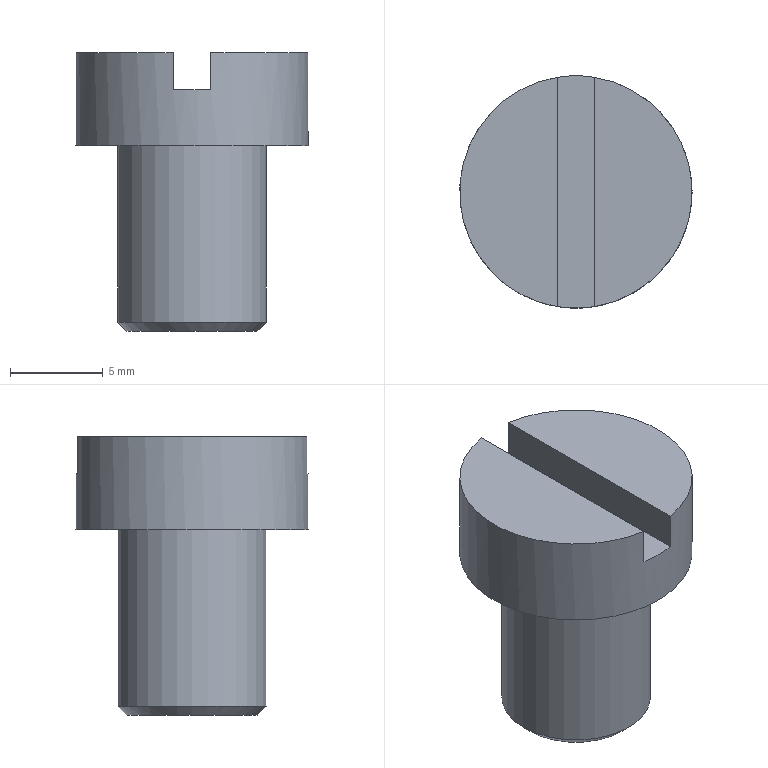Part | NX | features DATUM_CSYS 4, EXTRUDE 3, SKETCH 3, CHAMFER 1 | 1 solid | 10 faces | box 12.5 x 12.5 x 15 mm | volume 1063 mm3 | plane 7 | cylinder 2 | cone 1 | commonest cylinder face diameters 8 x1 12.5 x1
STEP:
#1=CARTESIAN_POINT('',(-1.,6.169,5.));
#2=VERTEX_POINT('',#1);
#3=CARTESIAN_POINT('',(-1.,-6.169,5.));
#4=VERTEX_POINT('',#3);
#5=CARTESIAN_POINT('',(-1.,13.407,5.));
#6=DIRECTION('',(0.,-1.,0.));
#7=VECTOR('',#6,1000.);
#8=LINE('',#5,#7);
#9=EDGE_CURVE('',#2,#4,#8,.T.);
#10=ORIENTED_EDGE('',*,*,#9,.F.);
#11=CARTESIAN_POINT('',(0.,0.,5.));
#12=DIRECTION('',(0.,0.,1.));
#13=DIRECTION('',(1.,0.,0.));
#14=AXIS2_PLACEMENT_3D('',#11,#12,#13);
#15=CIRCLE('',#14,6.25);
#16=EDGE_CURVE('',#2,#4,#15,.T.);
#17=ORIENTED_EDGE('',*,*,#16,.T.);
#18=EDGE_LOOP('',(#10,#17));
#19=FACE_BOUND('',#18,.T.);
#20=CARTESIAN_POINT('',(0.,0.,5.));
#21=DIRECTION('',(0.,0.,1.));
#22=DIRECTION('',(1.,0.,0.));
#23=AXIS2_PLACEMENT_3D('',#20,#21,#22);
#24=PLANE('',#23);
#25=ADVANCED_FACE('',(#19),#24,.T.);
#26=ORIENTED_EDGE('',*,*,#16,.F.);
#27=CARTESIAN_POINT('',(-1.,6.169,3.));
#28=VERTEX_POINT('',#27);
#29=CARTESIAN_POINT('',(-1.,6.169,5.));
#30=DIRECTION('',(0.,0.,-1.));
#31=VECTOR('',#30,1000.);
#32=LINE('',#29,#31);
#33=EDGE_CURVE('',#2,#28,#32,.T.);
#34=ORIENTED_EDGE('',*,*,#33,.T.);
#35=CARTESIAN_POINT('',(1.,6.169,3.));
#36=VERTEX_POINT('',#35);
#37=CARTESIAN_POINT('',(0.,0.,3.));
#38=DIRECTION('',(0.,0.,1.));
#39=DIRECTION('',(1.,0.,0.));
#40=AXIS2_PLACEMENT_3D('',#37,#38,#39);
#41=CIRCLE('',#40,6.25);
#42=EDGE_CURVE('',#36,#28,#41,.T.);
#43=ORIENTED_EDGE('',*,*,#42,.F.);
#44=CARTESIAN_POINT('',(1.,6.169,5.));
#45=VERTEX_POINT('',#44);
#46=CARTESIAN_POINT('',(1.,6.169,5.));
#47=DIRECTION('',(0.,0.,-1.));
#48=VECTOR('',#47,1000.);
#49=LINE('',#46,#48);
#50=EDGE_CURVE('',#36,#45,#49,.F.);
#51=ORIENTED_EDGE('',*,*,#50,.T.);
#52=CARTESIAN_POINT('',(1.,-6.169,5.));
#53=VERTEX_POINT('',#52);
#54=CARTESIAN_POINT('',(0.,0.,5.));
#55=DIRECTION('',(0.,0.,1.));
#56=DIRECTION('',(1.,0.,0.));
#57=AXIS2_PLACEMENT_3D('',#54,#55,#56);
#58=CIRCLE('',#57,6.25);
#59=EDGE_CURVE('',#53,#45,#58,.T.);
#60=ORIENTED_EDGE('',*,*,#59,.F.);
#61=CARTESIAN_POINT('',(1.,-6.169,3.));
#62=VERTEX_POINT('',#61);
#63=CARTESIAN_POINT('',(1.,-6.169,5.));
#64=DIRECTION('',(0.,0.,-1.));
#65=VECTOR('',#64,1000.);
#66=LINE('',#63,#65);
#67=EDGE_CURVE('',#53,#62,#66,.T.);
#68=ORIENTED_EDGE('',*,*,#67,.T.);
#69=CARTESIAN_POINT('',(-1.,-6.169,3.));
#70=VERTEX_POINT('',#69);
#71=CARTESIAN_POINT('',(0.,0.,3.));
#72=DIRECTION('',(0.,0.,1.));
#73=DIRECTION('',(1.,0.,0.));
#74=AXIS2_PLACEMENT_3D('',#71,#72,#73);
#75=CIRCLE('',#74,6.25);
#76=EDGE_CURVE('',#70,#62,#75,.T.);
#77=ORIENTED_EDGE('',*,*,#76,.F.);
#78=CARTESIAN_POINT('',(-1.,-6.169,5.));
#79=DIRECTION('',(0.,0.,-1.));
#80=VECTOR('',#79,1000.);
#81=LINE('',#78,#80);
#82=EDGE_CURVE('',#70,#4,#81,.F.);
#83=ORIENTED_EDGE('',*,*,#82,.T.);
#84=EDGE_LOOP('',(#26,#34,#43,#51,#60,#68,#77,#83));
#85=FACE_BOUND('',#84,.T.);
#86=CARTESIAN_POINT('',(6.25,0.,0.));
#87=VERTEX_POINT('',#86);
#88=CARTESIAN_POINT('',(0.,0.,0.));
#89=DIRECTION('',(0.,0.,1.));
#90=DIRECTION('',(1.,0.,0.));
#91=AXIS2_PLACEMENT_3D('',#88,#89,#90);
#92=CIRCLE('',#91,6.25);
#93=EDGE_CURVE('',#87,#87,#92,.T.);
#94=ORIENTED_EDGE('',*,*,#93,.T.);
#95=EDGE_LOOP('',(#94));
#96=FACE_BOUND('',#95,.T.);
#97=CARTESIAN_POINT('',(0.,0.,5.));
#98=DIRECTION('',(0.,0.,-1.));
#99=DIRECTION('',(-1.,0.,0.));
#100=AXIS2_PLACEMENT_3D('',#97,#98,#99);
#101=CYLINDRICAL_SURFACE('',#100,6.25);
#102=ADVANCED_FACE('',(#85,#96),#101,.T.);
#103=CARTESIAN_POINT('',(1.,-9.077,5.));
#104=DIRECTION('',(0.,1.,0.));
#105=VECTOR('',#104,1000.);
#106=LINE('',#103,#105);
#107=EDGE_CURVE('',#53,#45,#106,.T.);
#108=ORIENTED_EDGE('',*,*,#107,.F.);
#109=ORIENTED_EDGE('',*,*,#59,.T.);
#110=EDGE_LOOP('',(#108,#109));
#111=FACE_BOUND('',#110,.T.);
#112=CARTESIAN_POINT('',(0.,0.,5.));
#113=DIRECTION('',(0.,0.,1.));
#114=DIRECTION('',(1.,0.,0.));
#115=AXIS2_PLACEMENT_3D('',#112,#113,#114);
#116=PLANE('',#115);
#117=ADVANCED_FACE('',(#111),#116,.T.);
#118=CARTESIAN_POINT('',(4.,0.,0.));
#119=VERTEX_POINT('',#118);
#120=CARTESIAN_POINT('',(0.,0.,0.));
#121=DIRECTION('',(0.,0.,-1.));
#122=DIRECTION('',(1.,0.,0.));
#123=AXIS2_PLACEMENT_3D('',#120,#121,#122);
#124=CIRCLE('',#123,4.);
#125=EDGE_CURVE('',#119,#119,#124,.T.);
#126=ORIENTED_EDGE('',*,*,#125,.F.);
#127=EDGE_LOOP('',(#126));
#128=FACE_BOUND('',#127,.T.);
#129=ORIENTED_EDGE('',*,*,#93,.F.);
#130=EDGE_LOOP('',(#129));
#131=FACE_BOUND('',#130,.T.);
#132=CARTESIAN_POINT('',(0.,0.,0.));
#133=DIRECTION('',(0.,0.,1.));
#134=DIRECTION('',(1.,0.,0.));
#135=AXIS2_PLACEMENT_3D('',#132,#133,#134);
#136=PLANE('',#135);
#137=ADVANCED_FACE('',(#128,#131),#136,.F.);
#138=CARTESIAN_POINT('',(-4.,0.,-9.5));
#139=VERTEX_POINT('',#138);
#140=CARTESIAN_POINT('',(0.,0.,-9.5));
#141=DIRECTION('',(0.,0.,-1.));
#142=DIRECTION('',(-1.,0.,0.));
#143=AXIS2_PLACEMENT_3D('',#140,#141,#142);
#144=CIRCLE('',#143,4.);
#145=EDGE_CURVE('',#139,#139,#144,.F.);
#146=ORIENTED_EDGE('',*,*,#145,.T.);
#147=EDGE_LOOP('',(#146));
#148=FACE_BOUND('',#147,.T.);
#149=ORIENTED_EDGE('',*,*,#125,.T.);
#150=EDGE_LOOP('',(#149));
#151=FACE_BOUND('',#150,.T.);
#152=CARTESIAN_POINT('',(0.,0.,-10.));
#153=DIRECTION('',(0.,0.,1.));
#154=DIRECTION('',(1.,0.,0.));
#155=AXIS2_PLACEMENT_3D('',#152,#153,#154);
#156=CYLINDRICAL_SURFACE('',#155,4.);
#157=ADVANCED_FACE('',(#148,#151),#156,.T.);
#158=CARTESIAN_POINT('',(-3.5,0.,-10.));
#159=VERTEX_POINT('',#158);
#160=CARTESIAN_POINT('',(0.,0.,-10.));
#161=DIRECTION('',(0.,0.,-1.));
#162=DIRECTION('',(-1.,0.,0.));
#163=AXIS2_PLACEMENT_3D('',#160,#161,#162);
#164=CIRCLE('',#163,3.5);
#165=EDGE_CURVE('',#159,#159,#164,.T.);
#166=ORIENTED_EDGE('',*,*,#165,.T.);
#167=EDGE_LOOP('',(#166));
#168=FACE_BOUND('',#167,.T.);
#169=CARTESIAN_POINT('',(0.,0.,-10.));
#170=DIRECTION('',(0.,0.,-1.));
#171=DIRECTION('',(-1.,0.,0.));
#172=AXIS2_PLACEMENT_3D('',#169,#170,#171);
#173=PLANE('',#172);
#174=ADVANCED_FACE('',(#168),#173,.T.);
#175=ORIENTED_EDGE('',*,*,#42,.T.);
#176=CARTESIAN_POINT('',(-1.,13.407,3.));
#177=DIRECTION('',(0.,-1.,0.));
#178=VECTOR('',#177,1000.);
#179=LINE('',#176,#178);
#180=EDGE_CURVE('',#70,#28,#179,.F.);
#181=ORIENTED_EDGE('',*,*,#180,.F.);
#182=ORIENTED_EDGE('',*,*,#76,.T.);
#183=CARTESIAN_POINT('',(1.,-9.077,3.));
#184=DIRECTION('',(0.,1.,0.));
#185=VECTOR('',#184,1000.);
#186=LINE('',#183,#185);
#187=EDGE_CURVE('',#36,#62,#186,.F.);
#188=ORIENTED_EDGE('',*,*,#187,.F.);
#189=EDGE_LOOP('',(#175,#181,#182,#188));
#190=FACE_BOUND('',#189,.T.);
#191=CARTESIAN_POINT('',(0.,0.,3.));
#192=DIRECTION('',(0.,0.,1.));
#193=DIRECTION('',(1.,0.,0.));
#194=AXIS2_PLACEMENT_3D('',#191,#192,#193);
#195=PLANE('',#194);
#196=ADVANCED_FACE('',(#190),#195,.T.);
#197=ORIENTED_EDGE('',*,*,#9,.T.);
#198=ORIENTED_EDGE('',*,*,#82,.F.);
#199=ORIENTED_EDGE('',*,*,#180,.T.);
#200=ORIENTED_EDGE('',*,*,#33,.F.);
#201=EDGE_LOOP('',(#197,#198,#199,#200));
#202=FACE_BOUND('',#201,.T.);
#203=CARTESIAN_POINT('',(-1.,13.407,3.));
#204=DIRECTION('',(-1.,0.,0.));
#205=DIRECTION('',(0.,-1.,0.));
#206=AXIS2_PLACEMENT_3D('',#203,#204,#205);
#207=PLANE('',#206);
#208=ADVANCED_FACE('',(#202),#207,.F.);
#209=ORIENTED_EDGE('',*,*,#107,.T.);
#210=ORIENTED_EDGE('',*,*,#50,.F.);
#211=ORIENTED_EDGE('',*,*,#187,.T.);
#212=ORIENTED_EDGE('',*,*,#67,.F.);
#213=EDGE_LOOP('',(#209,#210,#211,#212));
#214=FACE_BOUND('',#213,.T.);
#215=CARTESIAN_POINT('',(1.,-9.077,3.));
#216=DIRECTION('',(1.,0.,0.));
#217=DIRECTION('',(0.,1.,0.));
#218=AXIS2_PLACEMENT_3D('',#215,#216,#217);
#219=PLANE('',#218);
#220=ADVANCED_FACE('',(#214),#219,.F.);
#221=ORIENTED_EDGE('',*,*,#145,.F.);
#222=EDGE_LOOP('',(#221));
#223=FACE_BOUND('',#222,.T.);
#224=ORIENTED_EDGE('',*,*,#165,.F.);
#225=EDGE_LOOP('',(#224));
#226=FACE_BOUND('',#225,.T.);
#227=CARTESIAN_POINT('',(0.,0.,-10.));
#228=DIRECTION('',(0.,0.,1.));
#229=DIRECTION('',(1.,0.,0.));
#230=AXIS2_PLACEMENT_3D('',#227,#228,#229);
#231=CONICAL_SURFACE('',#230,3.5,0.7854);
#232=ADVANCED_FACE('',(#223,#226),#231,.T.);
#233=CLOSED_SHELL('',(#25,#102,#117,#137,#157,#174,#196,#208,#220,#232));
#234=MANIFOLD_SOLID_BREP('',#233);
#235=(LENGTH_UNIT()NAMED_UNIT(*)SI_UNIT(.MILLI.,.METRE.));
#236=UNCERTAINTY_MEASURE_WITH_UNIT(LENGTH_MEASURE(0.00001),#235,'','');
#237=(NAMED_UNIT(*)PLANE_ANGLE_UNIT()SI_UNIT($,.RADIAN.));
#238=(NAMED_UNIT(*)SI_UNIT($,.STERADIAN.)SOLID_ANGLE_UNIT());
#239=(GEOMETRIC_REPRESENTATION_CONTEXT(3)GLOBAL_UNCERTAINTY_ASSIGNED_CONTEXT((#236))GLOBAL_UNIT_ASSIGNED_CONTEXT((#235,#237,#238))REPRESENTATION_CONTEXT('',''));
#240=ADVANCED_BREP_SHAPE_REPRESENTATION('',(#234),#239);